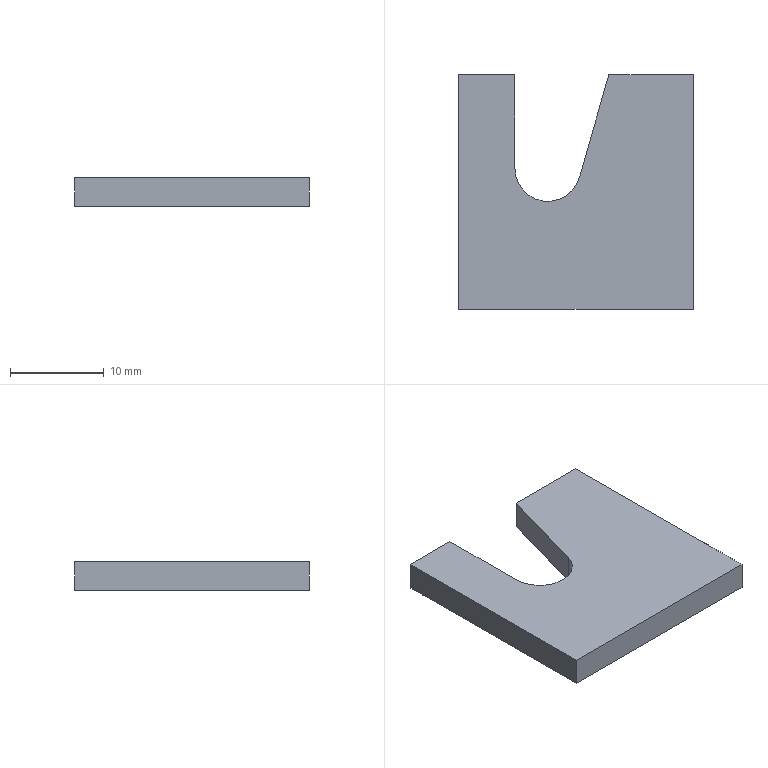Part | SolidWorks | features BaseBody 1 | 1 solid | 10 faces | box 25 x 25 x 3 mm | volume 1560 mm3 | plane 9 | cylinder 1 | commonest cylinder face diameters 7 x1
STEP:
#1=CARTESIAN_POINT('',(3.5,12.5,-3.));
#2=VERTEX_POINT('',#1);
#3=CARTESIAN_POINT('',(3.5,12.5,0.));
#4=VERTEX_POINT('',#3);
#5=CARTESIAN_POINT('',(3.5,12.5,-3.));
#6=DIRECTION('',(0.,0.,1.));
#7=VECTOR('',#6,1000.);
#8=LINE('',#5,#7);
#9=EDGE_CURVE('',#2,#4,#8,.T.);
#10=ORIENTED_EDGE('',*,*,#9,.F.);
#11=CARTESIAN_POINT('',(0.3651,1.538,-3.));
#12=VERTEX_POINT('',#11);
#13=CARTESIAN_POINT('',(-0.06898,0.01973,-3.));
#14=DIRECTION('',(0.2749,0.9615,0.));
#15=VECTOR('',#14,1000.);
#16=LINE('',#13,#15);
#17=EDGE_CURVE('',#12,#2,#16,.T.);
#18=ORIENTED_EDGE('',*,*,#17,.F.);
#19=CARTESIAN_POINT('',(0.3651,1.538,0.));
#20=VERTEX_POINT('',#19);
#21=CARTESIAN_POINT('',(0.3651,1.538,-3.));
#22=DIRECTION('',(0.,0.,1.));
#23=VECTOR('',#22,1000.);
#24=LINE('',#21,#23);
#25=EDGE_CURVE('',#12,#20,#24,.T.);
#26=ORIENTED_EDGE('',*,*,#25,.T.);
#27=CARTESIAN_POINT('',(-0.06898,0.01973,0.));
#28=DIRECTION('',(0.2749,0.9615,0.));
#29=VECTOR('',#28,1000.);
#30=LINE('',#27,#29);
#31=EDGE_CURVE('',#20,#4,#30,.T.);
#32=ORIENTED_EDGE('',*,*,#31,.T.);
#33=EDGE_LOOP('',(#10,#18,#26,#32));
#34=FACE_OUTER_BOUND('',#33,.T.);
#35=CARTESIAN_POINT('',(-0.06898,0.01973,-3.));
#36=DIRECTION('',(0.9615,-0.2749,0.));
#37=DIRECTION('',(0.,0.,-1.));
#38=AXIS2_PLACEMENT_3D('',#35,#36,#37);
#39=PLANE('',#38);
#40=ADVANCED_FACE('',(#34),#39,.F.);
#41=CARTESIAN_POINT('',(-6.5,12.5,-3.));
#42=VERTEX_POINT('',#41);
#43=CARTESIAN_POINT('',(-6.5,12.5,0.));
#44=VERTEX_POINT('',#43);
#45=CARTESIAN_POINT('',(-6.5,12.5,-10.));
#46=DIRECTION('',(0.,0.,1.));
#47=VECTOR('',#46,1000.);
#48=LINE('',#45,#47);
#49=EDGE_CURVE('',#42,#44,#48,.T.);
#50=ORIENTED_EDGE('',*,*,#49,.T.);
#51=CARTESIAN_POINT('',(-6.5,2.5,0.));
#52=VERTEX_POINT('',#51);
#53=CARTESIAN_POINT('',(-6.5,12.5,0.));
#54=DIRECTION('',(0.,-1.,0.));
#55=VECTOR('',#54,1000.);
#56=LINE('',#53,#55);
#57=EDGE_CURVE('',#44,#52,#56,.T.);
#58=ORIENTED_EDGE('',*,*,#57,.T.);
#59=CARTESIAN_POINT('',(-6.5,2.5,-3.));
#60=VERTEX_POINT('',#59);
#61=CARTESIAN_POINT('',(-6.5,2.5,-10.));
#62=DIRECTION('',(0.,0.,1.));
#63=VECTOR('',#62,1000.);
#64=LINE('',#61,#63);
#65=EDGE_CURVE('',#60,#52,#64,.T.);
#66=ORIENTED_EDGE('',*,*,#65,.F.);
#67=CARTESIAN_POINT('',(-6.5,0.,-3.));
#68=DIRECTION('',(0.,-1.,0.));
#69=VECTOR('',#68,1000.);
#70=LINE('',#67,#69);
#71=EDGE_CURVE('',#42,#60,#70,.T.);
#72=ORIENTED_EDGE('',*,*,#71,.F.);
#73=EDGE_LOOP('',(#50,#58,#66,#72));
#74=FACE_OUTER_BOUND('',#73,.T.);
#75=CARTESIAN_POINT('',(-6.5,12.5,-10.));
#76=DIRECTION('',(-1.,0.,0.));
#77=DIRECTION('',(0.,1.,0.));
#78=AXIS2_PLACEMENT_3D('',#75,#76,#77);
#79=PLANE('',#78);
#80=ADVANCED_FACE('',(#74),#79,.F.);
#81=ORIENTED_EDGE('',*,*,#49,.F.);
#82=CARTESIAN_POINT('',(-12.5,12.5,-3.));
#83=VERTEX_POINT('',#82);
#84=CARTESIAN_POINT('',(-12.5,12.5,-3.));
#85=DIRECTION('',(-1.,0.,0.));
#86=VECTOR('',#85,1000.);
#87=LINE('',#84,#86);
#88=EDGE_CURVE('',#42,#83,#87,.T.);
#89=ORIENTED_EDGE('',*,*,#88,.T.);
#90=CARTESIAN_POINT('',(-12.5,12.5,0.));
#91=VERTEX_POINT('',#90);
#92=CARTESIAN_POINT('',(-12.5,12.5,-3.));
#93=DIRECTION('',(0.,0.,1.));
#94=VECTOR('',#93,1000.);
#95=LINE('',#92,#94);
#96=EDGE_CURVE('',#83,#91,#95,.T.);
#97=ORIENTED_EDGE('',*,*,#96,.T.);
#98=CARTESIAN_POINT('',(-12.5,12.5,0.));
#99=DIRECTION('',(-1.,0.,0.));
#100=VECTOR('',#99,1000.);
#101=LINE('',#98,#100);
#102=EDGE_CURVE('',#44,#91,#101,.T.);
#103=ORIENTED_EDGE('',*,*,#102,.F.);
#104=EDGE_LOOP('',(#81,#89,#97,#103));
#105=FACE_OUTER_BOUND('',#104,.T.);
#106=CARTESIAN_POINT('',(-12.5,12.5,-3.));
#107=DIRECTION('',(0.,1.,0.));
#108=DIRECTION('',(1.,0.,0.));
#109=AXIS2_PLACEMENT_3D('',#106,#107,#108);
#110=PLANE('',#109);
#111=ADVANCED_FACE('',(#105),#110,.T.);
#112=CARTESIAN_POINT('',(-12.5,-12.5,0.));
#113=VERTEX_POINT('',#112);
#114=CARTESIAN_POINT('',(-12.5,12.5,0.));
#115=DIRECTION('',(0.,-1.,0.));
#116=VECTOR('',#115,1000.);
#117=LINE('',#114,#116);
#118=EDGE_CURVE('',#91,#113,#117,.T.);
#119=ORIENTED_EDGE('',*,*,#118,.F.);
#120=ORIENTED_EDGE('',*,*,#96,.F.);
#121=CARTESIAN_POINT('',(-12.5,-12.5,-3.));
#122=VERTEX_POINT('',#121);
#123=CARTESIAN_POINT('',(-12.5,12.5,-3.));
#124=DIRECTION('',(0.,-1.,0.));
#125=VECTOR('',#124,1000.);
#126=LINE('',#123,#125);
#127=EDGE_CURVE('',#83,#122,#126,.T.);
#128=ORIENTED_EDGE('',*,*,#127,.T.);
#129=CARTESIAN_POINT('',(-12.5,-12.5,-3.));
#130=DIRECTION('',(0.,0.,1.));
#131=VECTOR('',#130,1000.);
#132=LINE('',#129,#131);
#133=EDGE_CURVE('',#122,#113,#132,.T.);
#134=ORIENTED_EDGE('',*,*,#133,.T.);
#135=EDGE_LOOP('',(#119,#120,#128,#134));
#136=FACE_OUTER_BOUND('',#135,.T.);
#137=CARTESIAN_POINT('',(-12.5,12.5,-3.));
#138=DIRECTION('',(-1.,0.,0.));
#139=DIRECTION('',(0.,1.,0.));
#140=AXIS2_PLACEMENT_3D('',#137,#138,#139);
#141=PLANE('',#140);
#142=ADVANCED_FACE('',(#136),#141,.T.);
#143=CARTESIAN_POINT('',(12.5,-12.5,0.));
#144=VERTEX_POINT('',#143);
#145=CARTESIAN_POINT('',(-12.5,-12.5,0.));
#146=DIRECTION('',(1.,0.,0.));
#147=VECTOR('',#146,1000.);
#148=LINE('',#145,#147);
#149=EDGE_CURVE('',#113,#144,#148,.T.);
#150=ORIENTED_EDGE('',*,*,#149,.F.);
#151=ORIENTED_EDGE('',*,*,#133,.F.);
#152=CARTESIAN_POINT('',(12.5,-12.5,-3.));
#153=VERTEX_POINT('',#152);
#154=CARTESIAN_POINT('',(-12.5,-12.5,-3.));
#155=DIRECTION('',(1.,0.,0.));
#156=VECTOR('',#155,1000.);
#157=LINE('',#154,#156);
#158=EDGE_CURVE('',#122,#153,#157,.T.);
#159=ORIENTED_EDGE('',*,*,#158,.T.);
#160=CARTESIAN_POINT('',(12.5,-12.5,-3.));
#161=DIRECTION('',(0.,0.,1.));
#162=VECTOR('',#161,1000.);
#163=LINE('',#160,#162);
#164=EDGE_CURVE('',#153,#144,#163,.T.);
#165=ORIENTED_EDGE('',*,*,#164,.T.);
#166=EDGE_LOOP('',(#150,#151,#159,#165));
#167=FACE_OUTER_BOUND('',#166,.T.);
#168=CARTESIAN_POINT('',(-12.5,-12.5,-3.));
#169=DIRECTION('',(0.,-1.,0.));
#170=DIRECTION('',(0.,0.,-1.));
#171=AXIS2_PLACEMENT_3D('',#168,#169,#170);
#172=PLANE('',#171);
#173=ADVANCED_FACE('',(#167),#172,.T.);
#174=CARTESIAN_POINT('',(12.5,12.5,0.));
#175=VERTEX_POINT('',#174);
#176=CARTESIAN_POINT('',(12.5,12.5,0.));
#177=DIRECTION('',(0.,1.,0.));
#178=VECTOR('',#177,1000.);
#179=LINE('',#176,#178);
#180=EDGE_CURVE('',#144,#175,#179,.T.);
#181=ORIENTED_EDGE('',*,*,#180,.F.);
#182=ORIENTED_EDGE('',*,*,#164,.F.);
#183=CARTESIAN_POINT('',(12.5,12.5,-3.));
#184=VERTEX_POINT('',#183);
#185=CARTESIAN_POINT('',(12.5,12.5,-3.));
#186=DIRECTION('',(0.,1.,0.));
#187=VECTOR('',#186,1000.);
#188=LINE('',#185,#187);
#189=EDGE_CURVE('',#153,#184,#188,.T.);
#190=ORIENTED_EDGE('',*,*,#189,.T.);
#191=CARTESIAN_POINT('',(12.5,12.5,-3.));
#192=DIRECTION('',(0.,0.,1.));
#193=VECTOR('',#192,1000.);
#194=LINE('',#191,#193);
#195=EDGE_CURVE('',#184,#175,#194,.T.);
#196=ORIENTED_EDGE('',*,*,#195,.T.);
#197=EDGE_LOOP('',(#181,#182,#190,#196));
#198=FACE_OUTER_BOUND('',#197,.T.);
#199=CARTESIAN_POINT('',(12.5,12.5,-3.));
#200=DIRECTION('',(1.,0.,0.));
#201=DIRECTION('',(0.,1.,0.));
#202=AXIS2_PLACEMENT_3D('',#199,#200,#201);
#203=PLANE('',#202);
#204=ADVANCED_FACE('',(#198),#203,.T.);
#205=ORIENTED_EDGE('',*,*,#25,.F.);
#206=CARTESIAN_POINT('',(-3.,2.5,-3.));
#207=DIRECTION('',(0.,0.,1.));
#208=DIRECTION('',(1.,0.,0.));
#209=AXIS2_PLACEMENT_3D('',#206,#207,#208);
#210=CIRCLE('',#209,3.5);
#211=EDGE_CURVE('',#60,#12,#210,.T.);
#212=ORIENTED_EDGE('',*,*,#211,.F.);
#213=ORIENTED_EDGE('',*,*,#65,.T.);
#214=CARTESIAN_POINT('',(-3.,2.5,0.));
#215=DIRECTION('',(0.,0.,1.));
#216=DIRECTION('',(1.,0.,0.));
#217=AXIS2_PLACEMENT_3D('',#214,#215,#216);
#218=CIRCLE('',#217,3.5);
#219=EDGE_CURVE('',#52,#20,#218,.T.);
#220=ORIENTED_EDGE('',*,*,#219,.T.);
#221=EDGE_LOOP('',(#205,#212,#213,#220));
#222=FACE_OUTER_BOUND('',#221,.T.);
#223=CARTESIAN_POINT('',(-3.,2.5,-10.));
#224=DIRECTION('',(0.,0.,1.));
#225=DIRECTION('',(1.,0.,0.));
#226=AXIS2_PLACEMENT_3D('',#223,#224,#225);
#227=CYLINDRICAL_SURFACE('',#226,3.5);
#228=ADVANCED_FACE('',(#222),#227,.F.);
#229=CARTESIAN_POINT('',(-12.5,12.5,0.));
#230=DIRECTION('',(-1.,0.,0.));
#231=VECTOR('',#230,1000.);
#232=LINE('',#229,#231);
#233=EDGE_CURVE('',#175,#4,#232,.T.);
#234=ORIENTED_EDGE('',*,*,#233,.T.);
#235=ORIENTED_EDGE('',*,*,#31,.F.);
#236=ORIENTED_EDGE('',*,*,#219,.F.);
#237=ORIENTED_EDGE('',*,*,#57,.F.);
#238=ORIENTED_EDGE('',*,*,#102,.T.);
#239=ORIENTED_EDGE('',*,*,#118,.T.);
#240=ORIENTED_EDGE('',*,*,#149,.T.);
#241=ORIENTED_EDGE('',*,*,#180,.T.);
#242=EDGE_LOOP('',(#234,#235,#236,#237,#238,#239,#240,#241));
#243=FACE_OUTER_BOUND('',#242,.T.);
#244=CARTESIAN_POINT('',(0.,0.,0.));
#245=DIRECTION('',(0.,0.,1.));
#246=DIRECTION('',(1.,0.,0.));
#247=AXIS2_PLACEMENT_3D('',#244,#245,#246);
#248=PLANE('',#247);
#249=ADVANCED_FACE('',(#243),#248,.T.);
#250=ORIENTED_EDGE('',*,*,#17,.T.);
#251=CARTESIAN_POINT('',(-12.5,12.5,-3.));
#252=DIRECTION('',(-1.,0.,0.));
#253=VECTOR('',#252,1000.);
#254=LINE('',#251,#253);
#255=EDGE_CURVE('',#184,#2,#254,.T.);
#256=ORIENTED_EDGE('',*,*,#255,.F.);
#257=ORIENTED_EDGE('',*,*,#189,.F.);
#258=ORIENTED_EDGE('',*,*,#158,.F.);
#259=ORIENTED_EDGE('',*,*,#127,.F.);
#260=ORIENTED_EDGE('',*,*,#88,.F.);
#261=ORIENTED_EDGE('',*,*,#71,.T.);
#262=ORIENTED_EDGE('',*,*,#211,.T.);
#263=EDGE_LOOP('',(#250,#256,#257,#258,#259,#260,#261,#262));
#264=FACE_OUTER_BOUND('',#263,.T.);
#265=CARTESIAN_POINT('',(0.,0.,-3.));
#266=DIRECTION('',(0.,0.,1.));
#267=DIRECTION('',(1.,0.,0.));
#268=AXIS2_PLACEMENT_3D('',#265,#266,#267);
#269=PLANE('',#268);
#270=ADVANCED_FACE('',(#264),#269,.F.);
#271=ORIENTED_EDGE('',*,*,#255,.T.);
#272=ORIENTED_EDGE('',*,*,#9,.T.);
#273=ORIENTED_EDGE('',*,*,#233,.F.);
#274=ORIENTED_EDGE('',*,*,#195,.F.);
#275=EDGE_LOOP('',(#271,#272,#273,#274));
#276=FACE_OUTER_BOUND('',#275,.T.);
#277=CARTESIAN_POINT('',(-12.5,12.5,-3.));
#278=DIRECTION('',(0.,1.,0.));
#279=DIRECTION('',(1.,0.,0.));
#280=AXIS2_PLACEMENT_3D('',#277,#278,#279);
#281=PLANE('',#280);
#282=ADVANCED_FACE('',(#276),#281,.T.);
#283=CLOSED_SHELL('',(#40,#80,#111,#142,#173,#204,#228,#249,#270,#282));
#284=MANIFOLD_SOLID_BREP('',#283);
#285=CARTESIAN_POINT('',(0.,0.,0.));
#286=DIRECTION('',(0.,0.,1.));
#287=DIRECTION('',(1.,0.,0.));
#288=AXIS2_PLACEMENT_3D('',#285,#286,#287);
#289=(LENGTH_UNIT()NAMED_UNIT(*)SI_UNIT(.MILLI.,.METRE.));
#290=UNCERTAINTY_MEASURE_WITH_UNIT(LENGTH_MEASURE(0.00001),#289,'','');
#291=(NAMED_UNIT(*)PLANE_ANGLE_UNIT()SI_UNIT($,.RADIAN.));
#292=(NAMED_UNIT(*)SI_UNIT($,.STERADIAN.)SOLID_ANGLE_UNIT());
#293=(GEOMETRIC_REPRESENTATION_CONTEXT(3)GLOBAL_UNCERTAINTY_ASSIGNED_CONTEXT((#290))GLOBAL_UNIT_ASSIGNED_CONTEXT((#289,#291,#292))REPRESENTATION_CONTEXT('',''));
#294=ADVANCED_BREP_SHAPE_REPRESENTATION('',(#284,#288),#293);